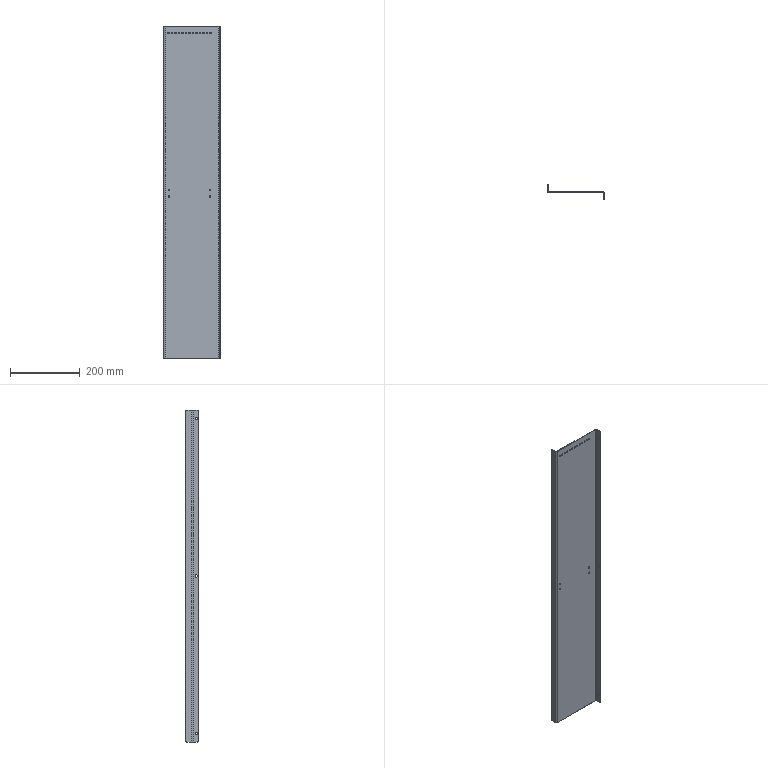Part | SolidWorks | features HoleWzd 3, Fillet 1, FlatPattern 1, SMBaseFlange 1, SheetMetal 1 | 1 solid | 66 faces | box 162 x 40 x 950 mm | volume 374388 mm3 | cylinder 48 | plane 18 | commonest cylinder face diameters 4.2 x34 6.6 x6 10 x4 4 x2 8 x2